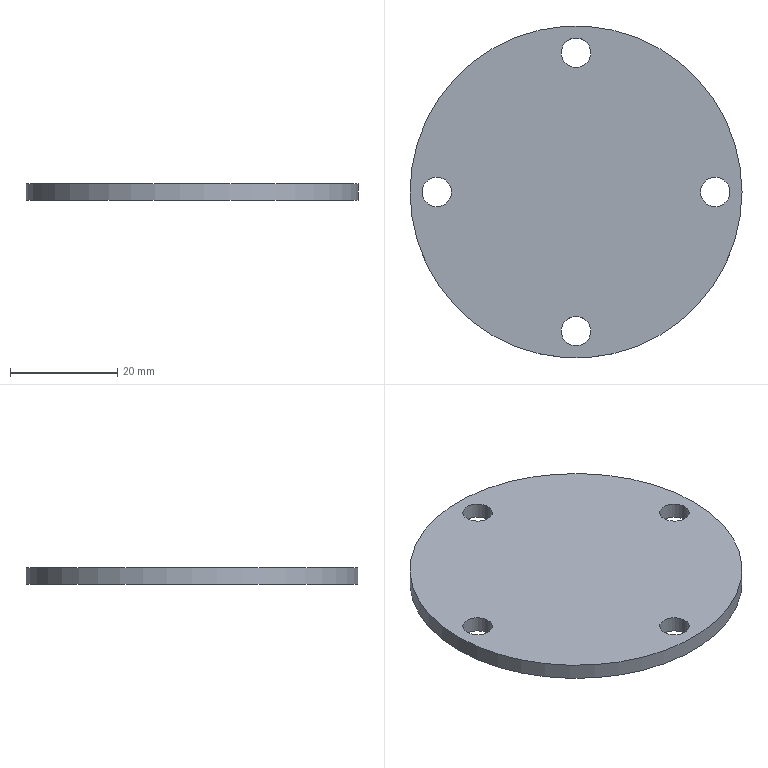Part | NX | features DATUM_CSYS 1, EXTRUDE 1, LINKED_FACE 1, SKETCH 1 | 1 solid | 7 faces | box 62 x 62 x 3 mm | volume 8772 mm3 | cylinder 5 | plane 2 | commonest cylinder face diameters 5.5 x4 62 x1
STEP:
#1=CARTESIAN_POINT('',(-2.75,26.,6.));
#2=VERTEX_POINT('',#1);
#3=CARTESIAN_POINT('',(0.,26.,6.));
#4=DIRECTION('',(0.,0.,-1.));
#5=DIRECTION('',(-1.,0.,0.));
#6=AXIS2_PLACEMENT_3D('',#3,#4,#5);
#7=CIRCLE('',#6,2.75);
#8=EDGE_CURVE('',#2,#2,#7,.T.);
#9=ORIENTED_EDGE('',*,*,#8,.F.);
#10=EDGE_LOOP('',(#9));
#11=FACE_BOUND('',#10,.T.);
#12=CARTESIAN_POINT('',(2.75,26.,3.));
#13=VERTEX_POINT('',#12);
#14=CARTESIAN_POINT('',(0.,26.,3.));
#15=DIRECTION('',(0.,0.,-1.));
#16=DIRECTION('',(1.,0.,0.));
#17=AXIS2_PLACEMENT_3D('',#14,#15,#16);
#18=CIRCLE('',#17,2.75);
#19=EDGE_CURVE('',#13,#13,#18,.T.);
#20=ORIENTED_EDGE('',*,*,#19,.T.);
#21=EDGE_LOOP('',(#20));
#22=FACE_BOUND('',#21,.T.);
#23=CARTESIAN_POINT('',(0.,26.,3.));
#24=DIRECTION('',(0.,0.,1.));
#25=DIRECTION('',(1.,0.,0.));
#26=AXIS2_PLACEMENT_3D('',#23,#24,#25);
#27=CYLINDRICAL_SURFACE('',#26,2.75);
#28=ADVANCED_FACE('',(#11,#22),#27,.F.);
#29=CARTESIAN_POINT('',(-2.75,-26.,6.));
#30=VERTEX_POINT('',#29);
#31=CARTESIAN_POINT('',(0.,-26.,6.));
#32=DIRECTION('',(0.,0.,-1.));
#33=DIRECTION('',(-1.,0.,0.));
#34=AXIS2_PLACEMENT_3D('',#31,#32,#33);
#35=CIRCLE('',#34,2.75);
#36=EDGE_CURVE('',#30,#30,#35,.T.);
#37=ORIENTED_EDGE('',*,*,#36,.F.);
#38=EDGE_LOOP('',(#37));
#39=FACE_BOUND('',#38,.T.);
#40=CARTESIAN_POINT('',(2.75,-26.,3.));
#41=VERTEX_POINT('',#40);
#42=CARTESIAN_POINT('',(0.,-26.,3.));
#43=DIRECTION('',(0.,0.,-1.));
#44=DIRECTION('',(1.,0.,0.));
#45=AXIS2_PLACEMENT_3D('',#42,#43,#44);
#46=CIRCLE('',#45,2.75);
#47=EDGE_CURVE('',#41,#41,#46,.T.);
#48=ORIENTED_EDGE('',*,*,#47,.T.);
#49=EDGE_LOOP('',(#48));
#50=FACE_BOUND('',#49,.T.);
#51=CARTESIAN_POINT('',(0.,-26.,3.));
#52=DIRECTION('',(0.,0.,1.));
#53=DIRECTION('',(1.,0.,0.));
#54=AXIS2_PLACEMENT_3D('',#51,#52,#53);
#55=CYLINDRICAL_SURFACE('',#54,2.75);
#56=ADVANCED_FACE('',(#39,#50),#55,.F.);
#57=CARTESIAN_POINT('',(-28.75,0.,6.));
#58=VERTEX_POINT('',#57);
#59=CARTESIAN_POINT('',(-26.,0.,6.));
#60=DIRECTION('',(0.,0.,-1.));
#61=DIRECTION('',(-1.,0.,0.));
#62=AXIS2_PLACEMENT_3D('',#59,#60,#61);
#63=CIRCLE('',#62,2.75);
#64=EDGE_CURVE('',#58,#58,#63,.T.);
#65=ORIENTED_EDGE('',*,*,#64,.F.);
#66=EDGE_LOOP('',(#65));
#67=FACE_BOUND('',#66,.T.);
#68=CARTESIAN_POINT('',(-23.25,0.,3.));
#69=VERTEX_POINT('',#68);
#70=CARTESIAN_POINT('',(-26.,0.,3.));
#71=DIRECTION('',(0.,0.,-1.));
#72=DIRECTION('',(1.,0.,0.));
#73=AXIS2_PLACEMENT_3D('',#70,#71,#72);
#74=CIRCLE('',#73,2.75);
#75=EDGE_CURVE('',#69,#69,#74,.T.);
#76=ORIENTED_EDGE('',*,*,#75,.T.);
#77=EDGE_LOOP('',(#76));
#78=FACE_BOUND('',#77,.T.);
#79=CARTESIAN_POINT('',(-26.,0.,3.));
#80=DIRECTION('',(0.,0.,1.));
#81=DIRECTION('',(1.,0.,0.));
#82=AXIS2_PLACEMENT_3D('',#79,#80,#81);
#83=CYLINDRICAL_SURFACE('',#82,2.75);
#84=ADVANCED_FACE('',(#67,#78),#83,.F.);
#85=CARTESIAN_POINT('',(-31.,0.,6.));
#86=VERTEX_POINT('',#85);
#87=CARTESIAN_POINT('',(0.,0.,6.));
#88=DIRECTION('',(0.,0.,1.));
#89=DIRECTION('',(-1.,0.,0.));
#90=AXIS2_PLACEMENT_3D('',#87,#88,#89);
#91=CIRCLE('',#90,31.);
#92=EDGE_CURVE('',#86,#86,#91,.T.);
#93=ORIENTED_EDGE('',*,*,#92,.F.);
#94=EDGE_LOOP('',(#93));
#95=FACE_BOUND('',#94,.T.);
#96=CARTESIAN_POINT('',(31.,0.,3.));
#97=VERTEX_POINT('',#96);
#98=CARTESIAN_POINT('',(0.,0.,3.));
#99=DIRECTION('',(0.,0.,1.));
#100=DIRECTION('',(1.,0.,0.));
#101=AXIS2_PLACEMENT_3D('',#98,#99,#100);
#102=CIRCLE('',#101,31.);
#103=EDGE_CURVE('',#97,#97,#102,.T.);
#104=ORIENTED_EDGE('',*,*,#103,.T.);
#105=EDGE_LOOP('',(#104));
#106=FACE_BOUND('',#105,.T.);
#107=CARTESIAN_POINT('',(0.,0.,3.));
#108=DIRECTION('',(0.,0.,1.));
#109=DIRECTION('',(1.,0.,0.));
#110=AXIS2_PLACEMENT_3D('',#107,#108,#109);
#111=CYLINDRICAL_SURFACE('',#110,31.);
#112=ADVANCED_FACE('',(#95,#106),#111,.T.);
#113=CARTESIAN_POINT('',(23.25,0.,6.));
#114=VERTEX_POINT('',#113);
#115=CARTESIAN_POINT('',(26.,0.,6.));
#116=DIRECTION('',(0.,0.,-1.));
#117=DIRECTION('',(-1.,0.,0.));
#118=AXIS2_PLACEMENT_3D('',#115,#116,#117);
#119=CIRCLE('',#118,2.75);
#120=EDGE_CURVE('',#114,#114,#119,.T.);
#121=ORIENTED_EDGE('',*,*,#120,.F.);
#122=EDGE_LOOP('',(#121));
#123=FACE_BOUND('',#122,.T.);
#124=CARTESIAN_POINT('',(28.75,0.,3.));
#125=VERTEX_POINT('',#124);
#126=CARTESIAN_POINT('',(26.,0.,3.));
#127=DIRECTION('',(0.,0.,-1.));
#128=DIRECTION('',(1.,0.,0.));
#129=AXIS2_PLACEMENT_3D('',#126,#127,#128);
#130=CIRCLE('',#129,2.75);
#131=EDGE_CURVE('',#125,#125,#130,.T.);
#132=ORIENTED_EDGE('',*,*,#131,.T.);
#133=EDGE_LOOP('',(#132));
#134=FACE_BOUND('',#133,.T.);
#135=CARTESIAN_POINT('',(26.,0.,3.));
#136=DIRECTION('',(0.,0.,1.));
#137=DIRECTION('',(1.,0.,0.));
#138=AXIS2_PLACEMENT_3D('',#135,#136,#137);
#139=CYLINDRICAL_SURFACE('',#138,2.75);
#140=ADVANCED_FACE('',(#123,#134),#139,.F.);
#141=ORIENTED_EDGE('',*,*,#103,.F.);
#142=EDGE_LOOP('',(#141));
#143=FACE_BOUND('',#142,.T.);
#144=ORIENTED_EDGE('',*,*,#75,.F.);
#145=EDGE_LOOP('',(#144));
#146=FACE_BOUND('',#145,.T.);
#147=ORIENTED_EDGE('',*,*,#47,.F.);
#148=EDGE_LOOP('',(#147));
#149=FACE_BOUND('',#148,.T.);
#150=ORIENTED_EDGE('',*,*,#19,.F.);
#151=EDGE_LOOP('',(#150));
#152=FACE_BOUND('',#151,.T.);
#153=ORIENTED_EDGE('',*,*,#131,.F.);
#154=EDGE_LOOP('',(#153));
#155=FACE_BOUND('',#154,.T.);
#156=CARTESIAN_POINT('',(-13.,0.,3.));
#157=DIRECTION('',(0.,0.,1.));
#158=DIRECTION('',(1.,0.,0.));
#159=AXIS2_PLACEMENT_3D('',#156,#157,#158);
#160=PLANE('',#159);
#161=ADVANCED_FACE('',(#143,#146,#149,#152,#155),#160,.F.);
#162=ORIENTED_EDGE('',*,*,#92,.T.);
#163=EDGE_LOOP('',(#162));
#164=FACE_BOUND('',#163,.T.);
#165=ORIENTED_EDGE('',*,*,#64,.T.);
#166=EDGE_LOOP('',(#165));
#167=FACE_BOUND('',#166,.T.);
#168=ORIENTED_EDGE('',*,*,#36,.T.);
#169=EDGE_LOOP('',(#168));
#170=FACE_BOUND('',#169,.T.);
#171=ORIENTED_EDGE('',*,*,#8,.T.);
#172=EDGE_LOOP('',(#171));
#173=FACE_BOUND('',#172,.T.);
#174=ORIENTED_EDGE('',*,*,#120,.T.);
#175=EDGE_LOOP('',(#174));
#176=FACE_BOUND('',#175,.T.);
#177=CARTESIAN_POINT('',(-13.,0.,6.));
#178=DIRECTION('',(0.,0.,1.));
#179=DIRECTION('',(1.,0.,0.));
#180=AXIS2_PLACEMENT_3D('',#177,#178,#179);
#181=PLANE('',#180);
#182=ADVANCED_FACE('',(#164,#167,#170,#173,#176),#181,.T.);
#183=CLOSED_SHELL('',(#28,#56,#84,#112,#140,#161,#182));
#184=MANIFOLD_SOLID_BREP('',#183);
#185=(LENGTH_UNIT()NAMED_UNIT(*)SI_UNIT(.MILLI.,.METRE.));
#186=UNCERTAINTY_MEASURE_WITH_UNIT(LENGTH_MEASURE(0.00001),#185,'','');
#187=(NAMED_UNIT(*)PLANE_ANGLE_UNIT()SI_UNIT($,.RADIAN.));
#188=(NAMED_UNIT(*)SI_UNIT($,.STERADIAN.)SOLID_ANGLE_UNIT());
#189=(GEOMETRIC_REPRESENTATION_CONTEXT(3)GLOBAL_UNCERTAINTY_ASSIGNED_CONTEXT((#186))GLOBAL_UNIT_ASSIGNED_CONTEXT((#185,#187,#188))REPRESENTATION_CONTEXT('',''));
#190=ADVANCED_BREP_SHAPE_REPRESENTATION('',(#184),#189);